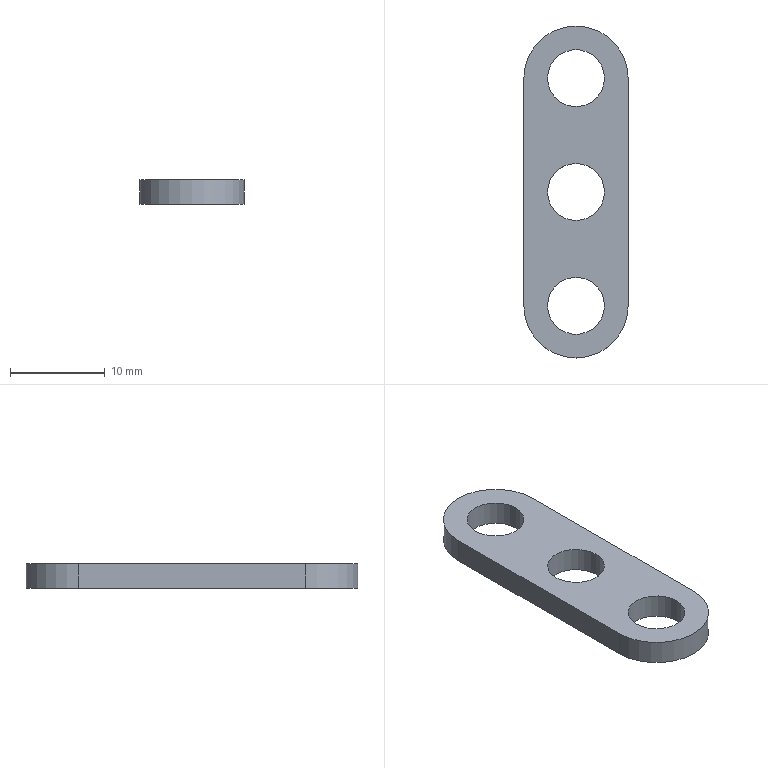Part | NX | features DATUM_CSYS 2, EXTRUDE 1, SKETCH 1 | 1 solid | 9 faces | box 11 x 35 x 2.6 mm | volume 712.946 mm3 | cylinder 5 | plane 4 | commonest cylinder face diameters 6 x3 11 x2
STEP:
#1=CARTESIAN_POINT('',(-5.5,12.,0.));
#2=VERTEX_POINT('',#1);
#3=CARTESIAN_POINT('',(-5.5,-12.,0.));
#4=VERTEX_POINT('',#3);
#5=CARTESIAN_POINT('',(-5.5,12.,0.));
#6=DIRECTION('',(0.,-1.,0.));
#7=VECTOR('',#6,1000.);
#8=LINE('',#5,#7);
#9=EDGE_CURVE('',#2,#4,#8,.T.);
#10=ORIENTED_EDGE('',*,*,#9,.T.);
#11=CARTESIAN_POINT('',(-5.5,-12.,2.6));
#12=VERTEX_POINT('',#11);
#13=CARTESIAN_POINT('',(-5.5,-12.,2.6));
#14=DIRECTION('',(0.,0.,-1.));
#15=VECTOR('',#14,1000.);
#16=LINE('',#13,#15);
#17=EDGE_CURVE('',#12,#4,#16,.T.);
#18=ORIENTED_EDGE('',*,*,#17,.F.);
#19=CARTESIAN_POINT('',(-5.5,12.,2.6));
#20=VERTEX_POINT('',#19);
#21=CARTESIAN_POINT('',(-5.5,12.,2.6));
#22=DIRECTION('',(0.,-1.,0.));
#23=VECTOR('',#22,1000.);
#24=LINE('',#21,#23);
#25=EDGE_CURVE('',#20,#12,#24,.T.);
#26=ORIENTED_EDGE('',*,*,#25,.F.);
#27=CARTESIAN_POINT('',(-5.5,12.,2.6));
#28=DIRECTION('',(0.,0.,-1.));
#29=VECTOR('',#28,1000.);
#30=LINE('',#27,#29);
#31=EDGE_CURVE('',#20,#2,#30,.T.);
#32=ORIENTED_EDGE('',*,*,#31,.T.);
#33=EDGE_LOOP('',(#10,#18,#26,#32));
#34=FACE_BOUND('',#33,.T.);
#35=CARTESIAN_POINT('',(-5.5,12.,2.6));
#36=DIRECTION('',(1.,0.,0.));
#37=DIRECTION('',(0.,0.,-1.));
#38=AXIS2_PLACEMENT_3D('',#35,#36,#37);
#39=PLANE('',#38);
#40=ADVANCED_FACE('',(#34),#39,.F.);
#41=CARTESIAN_POINT('',(5.5,-12.,0.));
#42=VERTEX_POINT('',#41);
#43=CARTESIAN_POINT('',(0.,-12.,0.));
#44=DIRECTION('',(0.,0.,1.));
#45=DIRECTION('',(1.,0.,0.));
#46=AXIS2_PLACEMENT_3D('',#43,#44,#45);
#47=CIRCLE('',#46,5.5);
#48=EDGE_CURVE('',#4,#42,#47,.T.);
#49=ORIENTED_EDGE('',*,*,#48,.T.);
#50=CARTESIAN_POINT('',(5.5,-12.,2.6));
#51=VERTEX_POINT('',#50);
#52=CARTESIAN_POINT('',(5.5,-12.,2.6));
#53=DIRECTION('',(0.,0.,-1.));
#54=VECTOR('',#53,1000.);
#55=LINE('',#52,#54);
#56=EDGE_CURVE('',#51,#42,#55,.T.);
#57=ORIENTED_EDGE('',*,*,#56,.F.);
#58=CARTESIAN_POINT('',(0.,-12.,2.6));
#59=DIRECTION('',(0.,0.,1.));
#60=DIRECTION('',(1.,0.,0.));
#61=AXIS2_PLACEMENT_3D('',#58,#59,#60);
#62=CIRCLE('',#61,5.5);
#63=EDGE_CURVE('',#12,#51,#62,.T.);
#64=ORIENTED_EDGE('',*,*,#63,.F.);
#65=ORIENTED_EDGE('',*,*,#17,.T.);
#66=EDGE_LOOP('',(#49,#57,#64,#65));
#67=FACE_BOUND('',#66,.T.);
#68=CARTESIAN_POINT('',(0.,-12.,2.6));
#69=DIRECTION('',(0.,0.,-1.));
#70=DIRECTION('',(-1.,0.,0.));
#71=AXIS2_PLACEMENT_3D('',#68,#69,#70);
#72=CYLINDRICAL_SURFACE('',#71,5.5);
#73=ADVANCED_FACE('',(#67),#72,.T.);
#74=CARTESIAN_POINT('',(5.5,12.,0.));
#75=VERTEX_POINT('',#74);
#76=CARTESIAN_POINT('',(5.5,-12.,0.));
#77=DIRECTION('',(0.,1.,0.));
#78=VECTOR('',#77,1000.);
#79=LINE('',#76,#78);
#80=EDGE_CURVE('',#42,#75,#79,.T.);
#81=ORIENTED_EDGE('',*,*,#80,.T.);
#82=CARTESIAN_POINT('',(5.5,12.,2.6));
#83=VERTEX_POINT('',#82);
#84=CARTESIAN_POINT('',(5.5,12.,2.6));
#85=DIRECTION('',(0.,0.,-1.));
#86=VECTOR('',#85,1000.);
#87=LINE('',#84,#86);
#88=EDGE_CURVE('',#83,#75,#87,.T.);
#89=ORIENTED_EDGE('',*,*,#88,.F.);
#90=CARTESIAN_POINT('',(5.5,-12.,2.6));
#91=DIRECTION('',(0.,1.,0.));
#92=VECTOR('',#91,1000.);
#93=LINE('',#90,#92);
#94=EDGE_CURVE('',#51,#83,#93,.T.);
#95=ORIENTED_EDGE('',*,*,#94,.F.);
#96=ORIENTED_EDGE('',*,*,#56,.T.);
#97=EDGE_LOOP('',(#81,#89,#95,#96));
#98=FACE_BOUND('',#97,.T.);
#99=CARTESIAN_POINT('',(5.5,-12.,2.6));
#100=DIRECTION('',(-1.,0.,0.));
#101=DIRECTION('',(0.,0.,1.));
#102=AXIS2_PLACEMENT_3D('',#99,#100,#101);
#103=PLANE('',#102);
#104=ADVANCED_FACE('',(#98),#103,.F.);
#105=CARTESIAN_POINT('',(3.,0.,2.6));
#106=VERTEX_POINT('',#105);
#107=CARTESIAN_POINT('',(0.,0.,2.6));
#108=DIRECTION('',(0.,0.,1.));
#109=DIRECTION('',(1.,0.,0.));
#110=AXIS2_PLACEMENT_3D('',#107,#108,#109);
#111=CIRCLE('',#110,3.);
#112=EDGE_CURVE('',#106,#106,#111,.T.);
#113=ORIENTED_EDGE('',*,*,#112,.T.);
#114=EDGE_LOOP('',(#113));
#115=FACE_BOUND('',#114,.T.);
#116=CARTESIAN_POINT('',(3.,0.,0.));
#117=VERTEX_POINT('',#116);
#118=CARTESIAN_POINT('',(0.,0.,0.));
#119=DIRECTION('',(0.,0.,1.));
#120=DIRECTION('',(1.,0.,0.));
#121=AXIS2_PLACEMENT_3D('',#118,#119,#120);
#122=CIRCLE('',#121,3.);
#123=EDGE_CURVE('',#117,#117,#122,.T.);
#124=ORIENTED_EDGE('',*,*,#123,.F.);
#125=EDGE_LOOP('',(#124));
#126=FACE_BOUND('',#125,.T.);
#127=CARTESIAN_POINT('',(0.,0.,2.6));
#128=DIRECTION('',(0.,0.,-1.));
#129=DIRECTION('',(-1.,0.,0.));
#130=AXIS2_PLACEMENT_3D('',#127,#128,#129);
#131=CYLINDRICAL_SURFACE('',#130,3.);
#132=ADVANCED_FACE('',(#115,#126),#131,.F.);
#133=CARTESIAN_POINT('',(3.,-12.,2.6));
#134=VERTEX_POINT('',#133);
#135=CARTESIAN_POINT('',(0.,-12.,2.6));
#136=DIRECTION('',(0.,0.,1.));
#137=DIRECTION('',(1.,0.,0.));
#138=AXIS2_PLACEMENT_3D('',#135,#136,#137);
#139=CIRCLE('',#138,3.);
#140=EDGE_CURVE('',#134,#134,#139,.T.);
#141=ORIENTED_EDGE('',*,*,#140,.T.);
#142=EDGE_LOOP('',(#141));
#143=FACE_BOUND('',#142,.T.);
#144=CARTESIAN_POINT('',(3.,-12.,0.));
#145=VERTEX_POINT('',#144);
#146=CARTESIAN_POINT('',(0.,-12.,0.));
#147=DIRECTION('',(0.,0.,1.));
#148=DIRECTION('',(1.,0.,0.));
#149=AXIS2_PLACEMENT_3D('',#146,#147,#148);
#150=CIRCLE('',#149,3.);
#151=EDGE_CURVE('',#145,#145,#150,.T.);
#152=ORIENTED_EDGE('',*,*,#151,.F.);
#153=EDGE_LOOP('',(#152));
#154=FACE_BOUND('',#153,.T.);
#155=CARTESIAN_POINT('',(0.,-12.,2.6));
#156=DIRECTION('',(0.,0.,-1.));
#157=DIRECTION('',(-1.,0.,0.));
#158=AXIS2_PLACEMENT_3D('',#155,#156,#157);
#159=CYLINDRICAL_SURFACE('',#158,3.);
#160=ADVANCED_FACE('',(#143,#154),#159,.F.);
#161=CARTESIAN_POINT('',(0.,12.,0.));
#162=DIRECTION('',(0.,0.,1.));
#163=DIRECTION('',(1.,0.,0.));
#164=AXIS2_PLACEMENT_3D('',#161,#162,#163);
#165=CIRCLE('',#164,5.5);
#166=EDGE_CURVE('',#75,#2,#165,.T.);
#167=ORIENTED_EDGE('',*,*,#166,.T.);
#168=ORIENTED_EDGE('',*,*,#31,.F.);
#169=CARTESIAN_POINT('',(0.,12.,2.6));
#170=DIRECTION('',(0.,0.,1.));
#171=DIRECTION('',(1.,0.,0.));
#172=AXIS2_PLACEMENT_3D('',#169,#170,#171);
#173=CIRCLE('',#172,5.5);
#174=EDGE_CURVE('',#83,#20,#173,.T.);
#175=ORIENTED_EDGE('',*,*,#174,.F.);
#176=ORIENTED_EDGE('',*,*,#88,.T.);
#177=EDGE_LOOP('',(#167,#168,#175,#176));
#178=FACE_BOUND('',#177,.T.);
#179=CARTESIAN_POINT('',(0.,12.,2.6));
#180=DIRECTION('',(0.,0.,-1.));
#181=DIRECTION('',(-1.,0.,0.));
#182=AXIS2_PLACEMENT_3D('',#179,#180,#181);
#183=CYLINDRICAL_SURFACE('',#182,5.5);
#184=ADVANCED_FACE('',(#178),#183,.T.);
#185=CARTESIAN_POINT('',(3.,12.,2.6));
#186=VERTEX_POINT('',#185);
#187=CARTESIAN_POINT('',(0.,12.,2.6));
#188=DIRECTION('',(0.,0.,1.));
#189=DIRECTION('',(1.,0.,0.));
#190=AXIS2_PLACEMENT_3D('',#187,#188,#189);
#191=CIRCLE('',#190,3.);
#192=EDGE_CURVE('',#186,#186,#191,.T.);
#193=ORIENTED_EDGE('',*,*,#192,.T.);
#194=EDGE_LOOP('',(#193));
#195=FACE_BOUND('',#194,.T.);
#196=CARTESIAN_POINT('',(3.,12.,0.));
#197=VERTEX_POINT('',#196);
#198=CARTESIAN_POINT('',(0.,12.,0.));
#199=DIRECTION('',(0.,0.,1.));
#200=DIRECTION('',(1.,0.,0.));
#201=AXIS2_PLACEMENT_3D('',#198,#199,#200);
#202=CIRCLE('',#201,3.);
#203=EDGE_CURVE('',#197,#197,#202,.T.);
#204=ORIENTED_EDGE('',*,*,#203,.F.);
#205=EDGE_LOOP('',(#204));
#206=FACE_BOUND('',#205,.T.);
#207=CARTESIAN_POINT('',(0.,12.,2.6));
#208=DIRECTION('',(0.,0.,-1.));
#209=DIRECTION('',(-1.,0.,0.));
#210=AXIS2_PLACEMENT_3D('',#207,#208,#209);
#211=CYLINDRICAL_SURFACE('',#210,3.);
#212=ADVANCED_FACE('',(#195,#206),#211,.F.);
#213=ORIENTED_EDGE('',*,*,#25,.T.);
#214=ORIENTED_EDGE('',*,*,#63,.T.);
#215=ORIENTED_EDGE('',*,*,#94,.T.);
#216=ORIENTED_EDGE('',*,*,#174,.T.);
#217=EDGE_LOOP('',(#213,#214,#215,#216));
#218=FACE_BOUND('',#217,.T.);
#219=ORIENTED_EDGE('',*,*,#140,.F.);
#220=EDGE_LOOP('',(#219));
#221=FACE_BOUND('',#220,.T.);
#222=ORIENTED_EDGE('',*,*,#112,.F.);
#223=EDGE_LOOP('',(#222));
#224=FACE_BOUND('',#223,.T.);
#225=ORIENTED_EDGE('',*,*,#192,.F.);
#226=EDGE_LOOP('',(#225));
#227=FACE_BOUND('',#226,.T.);
#228=CARTESIAN_POINT('',(0.,-12.,2.6));
#229=DIRECTION('',(0.,0.,1.));
#230=DIRECTION('',(1.,0.,0.));
#231=AXIS2_PLACEMENT_3D('',#228,#229,#230);
#232=PLANE('',#231);
#233=ADVANCED_FACE('',(#218,#221,#224,#227),#232,.T.);
#234=ORIENTED_EDGE('',*,*,#9,.F.);
#235=ORIENTED_EDGE('',*,*,#166,.F.);
#236=ORIENTED_EDGE('',*,*,#80,.F.);
#237=ORIENTED_EDGE('',*,*,#48,.F.);
#238=EDGE_LOOP('',(#234,#235,#236,#237));
#239=FACE_BOUND('',#238,.T.);
#240=ORIENTED_EDGE('',*,*,#151,.T.);
#241=EDGE_LOOP('',(#240));
#242=FACE_BOUND('',#241,.T.);
#243=ORIENTED_EDGE('',*,*,#123,.T.);
#244=EDGE_LOOP('',(#243));
#245=FACE_BOUND('',#244,.T.);
#246=ORIENTED_EDGE('',*,*,#203,.T.);
#247=EDGE_LOOP('',(#246));
#248=FACE_BOUND('',#247,.T.);
#249=CARTESIAN_POINT('',(0.,-12.,0.));
#250=DIRECTION('',(0.,0.,1.));
#251=DIRECTION('',(1.,0.,0.));
#252=AXIS2_PLACEMENT_3D('',#249,#250,#251);
#253=PLANE('',#252);
#254=ADVANCED_FACE('',(#239,#242,#245,#248),#253,.F.);
#255=CLOSED_SHELL('',(#40,#73,#104,#132,#160,#184,#212,#233,#254));
#256=MANIFOLD_SOLID_BREP('',#255);
#257=(LENGTH_UNIT()NAMED_UNIT(*)SI_UNIT(.MILLI.,.METRE.));
#258=UNCERTAINTY_MEASURE_WITH_UNIT(LENGTH_MEASURE(0.00001),#257,'','');
#259=(NAMED_UNIT(*)PLANE_ANGLE_UNIT()SI_UNIT($,.RADIAN.));
#260=(NAMED_UNIT(*)SI_UNIT($,.STERADIAN.)SOLID_ANGLE_UNIT());
#261=(GEOMETRIC_REPRESENTATION_CONTEXT(3)GLOBAL_UNCERTAINTY_ASSIGNED_CONTEXT((#258))GLOBAL_UNIT_ASSIGNED_CONTEXT((#257,#259,#260))REPRESENTATION_CONTEXT('',''));
#262=ADVANCED_BREP_SHAPE_REPRESENTATION('',(#256),#261);